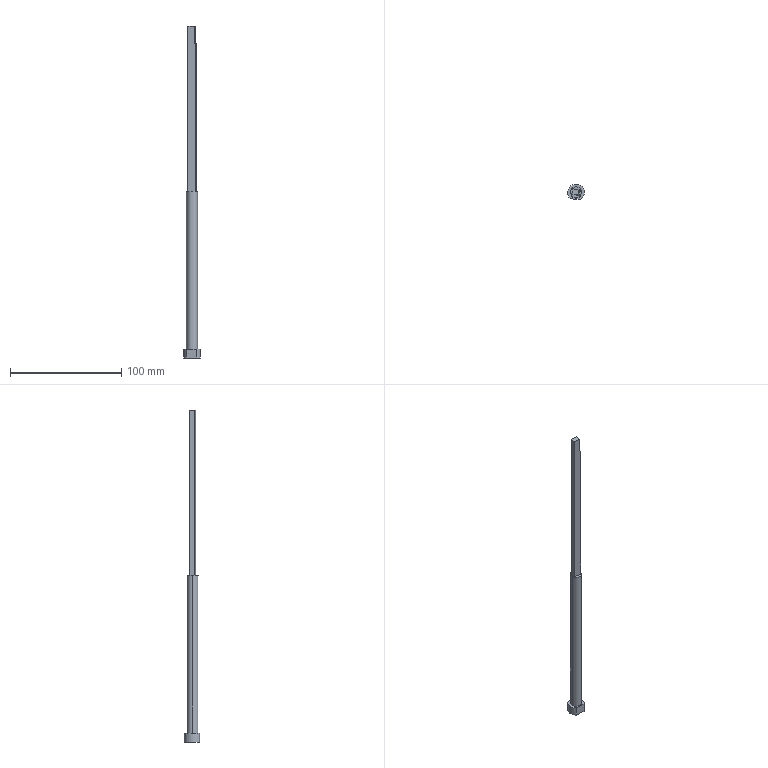Part | Creo | 1 solid | 14 faces | box 15 x 13.938 x 298.951 mm | volume 17637 mm3 | plane 10 | cylinder 3 | cone 1 | commonest cylinder face diameters 10 x2 15 x1
STEP:
#1=CARTESIAN_POINT('',(-71.051,51.227,-12.688));
#2=VERTEX_POINT('',#1);
#3=CARTESIAN_POINT('',(-71.051,51.227,-146.));
#4=VERTEX_POINT('',#3);
#5=CARTESIAN_POINT('',(-71.051,51.227,-12.688));
#6=DIRECTION('',(0.,0.,-1.));
#7=VECTOR('',#6,133.312);
#8=LINE('',#5,#7);
#9=EDGE_CURVE('',#2,#4,#8,.T.);
#10=ORIENTED_EDGE('',*,*,#9,.F.);
#11=CARTESIAN_POINT('',(-70.529,56.199,-12.688));
#12=VERTEX_POINT('',#11);
#13=CARTESIAN_POINT('',(-71.051,51.227,-12.688));
#14=DIRECTION('',(0.1045,0.9945,0.));
#15=VECTOR('',#14,5.);
#16=LINE('',#13,#15);
#17=EDGE_CURVE('',#2,#12,#16,.T.);
#18=ORIENTED_EDGE('',*,*,#17,.T.);
#19=CARTESIAN_POINT('',(-70.529,56.199,-146.));
#20=VERTEX_POINT('',#19);
#21=CARTESIAN_POINT('',(-70.529,56.199,-12.688));
#22=DIRECTION('',(0.,0.,-1.));
#23=VECTOR('',#22,133.312);
#24=LINE('',#21,#23);
#25=EDGE_CURVE('',#12,#20,#24,.T.);
#26=ORIENTED_EDGE('',*,*,#25,.T.);
#27=CARTESIAN_POINT('',(-70.529,56.199,-146.));
#28=DIRECTION('',(-0.1045,-0.9945,0.));
#29=VECTOR('',#28,5.);
#30=LINE('',#27,#29);
#31=EDGE_CURVE('',#20,#4,#30,.T.);
#32=ORIENTED_EDGE('',*,*,#31,.T.);
#33=EDGE_LOOP('',(#10,#18,#26,#32));
#34=FACE_OUTER_BOUND('',#33,.F.);
#35=CARTESIAN_POINT('',(-70.921,52.47,-35.));
#36=DIRECTION('',(0.9945,-0.1045,0.));
#37=DIRECTION('',(0.,0.,1.));
#38=AXIS2_PLACEMENT_3D('',#35,#36,#37);
#39=PLANE('',#38);
#40=ADVANCED_FACE('',(#34),#39,.T.);
#41=CARTESIAN_POINT('',(-71.854,51.311,-12.688));
#42=VERTEX_POINT('',#41);
#43=CARTESIAN_POINT('',(-72.124,51.34,2.9));
#44=VERTEX_POINT('',#43);
#45=CARTESIAN_POINT('',(-71.854,51.311,-12.688));
#46=DIRECTION('',(-0.01736,0.001825,0.9998));
#47=VECTOR('',#46,15.59);
#48=LINE('',#45,#47);
#49=EDGE_CURVE('',#42,#44,#48,.T.);
#50=ORIENTED_EDGE('',*,*,#49,.F.);
#51=CARTESIAN_POINT('',(-71.854,51.311,-12.688));
#52=DIRECTION('',(0.9945,-0.1045,-0.000006119));
#53=VECTOR('',#52,0.807);
#54=LINE('',#51,#53);
#55=EDGE_CURVE('',#42,#2,#54,.T.);
#56=ORIENTED_EDGE('',*,*,#55,.T.);
#57=ORIENTED_EDGE('',*,*,#9,.T.);
#58=CARTESIAN_POINT('',(-78.013,51.958,-146.));
#59=VERTEX_POINT('',#58);
#60=CARTESIAN_POINT('',(-71.051,51.227,-146.));
#61=DIRECTION('',(-0.9945,0.1045,0.));
#62=VECTOR('',#61,7.);
#63=LINE('',#60,#62);
#64=EDGE_CURVE('',#4,#59,#63,.T.);
#65=ORIENTED_EDGE('',*,*,#64,.T.);
#66=CARTESIAN_POINT('',(-78.013,51.958,2.951));
#67=VERTEX_POINT('',#66);
#68=CARTESIAN_POINT('',(-78.013,51.958,2.951));
#69=DIRECTION('',(0.,0.,-1.));
#70=VECTOR('',#69,148.951);
#71=LINE('',#68,#70);
#72=EDGE_CURVE('',#67,#59,#71,.T.);
#73=ORIENTED_EDGE('',*,*,#72,.F.);
#74=CARTESIAN_POINT('',(-78.013,51.958,2.951));
#75=DIRECTION('',(0.9945,-0.1045,-0.008677));
#76=VECTOR('',#75,5.921);
#77=LINE('',#74,#76);
#78=EDGE_CURVE('',#67,#44,#77,.T.);
#79=ORIENTED_EDGE('',*,*,#78,.T.);
#80=EDGE_LOOP('',(#50,#56,#57,#65,#73,#79));
#81=FACE_OUTER_BOUND('',#80,.F.);
#82=CARTESIAN_POINT('',(-75.775,51.723,-35.));
#83=DIRECTION('',(-0.1045,-0.9945,0.));
#84=DIRECTION('',(0.,0.,1.));
#85=AXIS2_PLACEMENT_3D('',#82,#83,#84);
#86=PLANE('',#85);
#87=ADVANCED_FACE('',(#81),#86,.T.);
#88=CARTESIAN_POINT('',(-71.456,56.297,2.894));
#89=VERTEX_POINT('',#88);
#90=CARTESIAN_POINT('',(-71.185,56.268,-12.688));
#91=VERTEX_POINT('',#90);
#92=CARTESIAN_POINT('',(-71.456,56.297,2.894));
#93=DIRECTION('',(0.01737,-0.001825,-0.9998));
#94=VECTOR('',#93,15.585);
#95=LINE('',#92,#94);
#96=EDGE_CURVE('',#89,#91,#95,.T.);
#97=ORIENTED_EDGE('',*,*,#96,.T.);
#98=CARTESIAN_POINT('',(-71.185,56.268,-12.688));
#99=CARTESIAN_POINT('',(-71.263,55.717,-12.688));
#100=CARTESIAN_POINT('',(-71.417,54.613,-12.688));
#101=CARTESIAN_POINT('',(-71.639,52.961,-12.688));
#102=CARTESIAN_POINT('',(-71.783,51.861,-12.688));
#103=CARTESIAN_POINT('',(-71.854,51.311,-12.688));
#104=B_SPLINE_CURVE_WITH_KNOTS('',3,(#98,#99,#100,#101,#102,#103),.UNSPECIFIED.,.F.,.F.,(4,1,1,4),(0.,0.3333,0.6667,1.),.UNSPECIFIED.);
#105=EDGE_CURVE('',#91,#42,#104,.T.);
#106=ORIENTED_EDGE('',*,*,#105,.T.);
#107=ORIENTED_EDGE('',*,*,#49,.T.);
#108=CARTESIAN_POINT('',(-72.124,51.34,2.9));
#109=CARTESIAN_POINT('',(-72.053,51.891,2.899));
#110=CARTESIAN_POINT('',(-71.91,52.993,2.898));
#111=CARTESIAN_POINT('',(-71.687,54.646,2.896));
#112=CARTESIAN_POINT('',(-71.533,55.746,2.895));
#113=CARTESIAN_POINT('',(-71.456,56.297,2.894));
#114=B_SPLINE_CURVE_WITH_KNOTS('',3,(#108,#109,#110,#111,#112,#113),.UNSPECIFIED.,.F.,.F.,(4,1,1,4),(0.,0.3333,0.6667,1.),.UNSPECIFIED.);
#115=EDGE_CURVE('',#44,#89,#114,.T.);
#116=ORIENTED_EDGE('',*,*,#115,.T.);
#117=EDGE_LOOP('',(#97,#106,#107,#116));
#118=FACE_OUTER_BOUND('',#117,.F.);
#119=CARTESIAN_POINT('',(344.456,-2.301,-4.943));
#120=DIRECTION('',(0.0001143,-0.00001653,1.));
#121=DIRECTION('',(-0.9902,0.1395,0.0001155));
#122=AXIS2_PLACEMENT_3D('',#119,#120,#121);
#123=CONICAL_SURFACE('',#122,419.883,1.007);
#124=ADVANCED_FACE('',(#118),#123,.F.);
#125=ORIENTED_EDGE('',*,*,#25,.F.);
#126=CARTESIAN_POINT('',(-70.529,56.199,-12.688));
#127=DIRECTION('',(-0.9945,0.1045,0.000007477));
#128=VECTOR('',#127,0.6604);
#129=LINE('',#126,#128);
#130=EDGE_CURVE('',#12,#91,#129,.T.);
#131=ORIENTED_EDGE('',*,*,#130,.T.);
#132=ORIENTED_EDGE('',*,*,#96,.F.);
#133=CARTESIAN_POINT('',(-77.49,56.931,2.947));
#134=VERTEX_POINT('',#133);
#135=CARTESIAN_POINT('',(-71.456,56.297,2.894));
#136=DIRECTION('',(-0.9945,0.1045,0.008678));
#137=VECTOR('',#136,6.068);
#138=LINE('',#135,#137);
#139=EDGE_CURVE('',#89,#134,#138,.T.);
#140=ORIENTED_EDGE('',*,*,#139,.T.);
#141=CARTESIAN_POINT('',(-77.49,56.931,-146.));
#142=VERTEX_POINT('',#141);
#143=CARTESIAN_POINT('',(-77.49,56.931,2.947));
#144=DIRECTION('',(0.,0.,-1.));
#145=VECTOR('',#144,148.947);
#146=LINE('',#143,#145);
#147=EDGE_CURVE('',#134,#142,#146,.T.);
#148=ORIENTED_EDGE('',*,*,#147,.T.);
#149=CARTESIAN_POINT('',(-77.49,56.931,-146.));
#150=DIRECTION('',(0.9945,-0.1045,0.));
#151=VECTOR('',#150,7.);
#152=LINE('',#149,#151);
#153=EDGE_CURVE('',#142,#20,#152,.T.);
#154=ORIENTED_EDGE('',*,*,#153,.T.);
#155=EDGE_LOOP('',(#125,#131,#132,#140,#148,#154));
#156=FACE_OUTER_BOUND('',#155,.F.);
#157=CARTESIAN_POINT('',(-75.253,56.696,-35.));
#158=DIRECTION('',(0.1045,0.9945,0.));
#159=DIRECTION('',(0.,0.,-1.));
#160=AXIS2_PLACEMENT_3D('',#157,#158,#159);
#161=PLANE('',#160);
#162=ADVANCED_FACE('',(#156),#161,.T.);
#163=ORIENTED_EDGE('',*,*,#17,.F.);
#164=ORIENTED_EDGE('',*,*,#55,.F.);
#165=ORIENTED_EDGE('',*,*,#105,.F.);
#166=ORIENTED_EDGE('',*,*,#130,.F.);
#167=EDGE_LOOP('',(#163,#164,#165,#166));
#168=FACE_OUTER_BOUND('',#167,.F.);
#169=CARTESIAN_POINT('',(0.,0.,-12.688));
#170=DIRECTION('',(0.,0.,1.));
#171=DIRECTION('',(0.,-1.,0.));
#172=AXIS2_PLACEMENT_3D('',#169,#170,#171);
#173=PLANE('',#172);
#174=ADVANCED_FACE('',(#168),#173,.T.);
#175=ORIENTED_EDGE('',*,*,#115,.F.);
#176=ORIENTED_EDGE('',*,*,#78,.F.);
#177=CARTESIAN_POINT('',(-77.49,56.931,2.947));
#178=DIRECTION('',(-0.1045,-0.9945,0.0009122));
#179=VECTOR('',#178,5.);
#180=LINE('',#177,#179);
#181=EDGE_CURVE('',#134,#67,#180,.T.);
#182=ORIENTED_EDGE('',*,*,#181,.F.);
#183=ORIENTED_EDGE('',*,*,#139,.F.);
#184=EDGE_LOOP('',(#175,#176,#182,#183));
#185=FACE_OUTER_BOUND('',#184,.F.);
#186=CARTESIAN_POINT('',(-86.668,59.295,3.027));
#187=DIRECTION('',(0.008727,0.,1.));
#188=DIRECTION('',(0.,-1.,0.));
#189=AXIS2_PLACEMENT_3D('',#186,#187,#188);
#190=PLANE('',#189);
#191=ADVANCED_FACE('',(#185),#190,.T.);
#192=ORIENTED_EDGE('',*,*,#147,.F.);
#193=ORIENTED_EDGE('',*,*,#181,.T.);
#194=ORIENTED_EDGE('',*,*,#72,.T.);
#195=CARTESIAN_POINT('',(-78.013,51.958,-146.));
#196=DIRECTION('',(0.1045,0.9945,0.));
#197=VECTOR('',#196,5.);
#198=LINE('',#195,#197);
#199=EDGE_CURVE('',#59,#142,#198,.T.);
#200=ORIENTED_EDGE('',*,*,#199,.T.);
#201=EDGE_LOOP('',(#192,#193,#194,#200));
#202=FACE_OUTER_BOUND('',#201,.F.);
#203=CARTESIAN_POINT('',(-77.882,53.202,-35.));
#204=DIRECTION('',(-0.9945,0.1045,0.));
#205=DIRECTION('',(0.,0.,-1.));
#206=AXIS2_PLACEMENT_3D('',#203,#204,#205);
#207=PLANE('',#206);
#208=ADVANCED_FACE('',(#202),#207,.T.);
#209=CARTESIAN_POINT('',(-69.271,54.079,-146.));
#210=VERTEX_POINT('',#209);
#211=CARTESIAN_POINT('',(-79.271,54.079,-146.));
#212=VERTEX_POINT('',#211);
#213=CARTESIAN_POINT('',(-74.271,54.079,-146.));
#214=DIRECTION('',(0.,0.,1.));
#215=DIRECTION('',(1.,0.,0.));
#216=AXIS2_PLACEMENT_3D('',#213,#214,#215);
#217=CIRCLE('',#216,5.);
#218=EDGE_CURVE('',#210,#212,#217,.T.);
#219=ORIENTED_EDGE('',*,*,#218,.F.);
#220=CARTESIAN_POINT('',(-74.271,54.079,-146.));
#221=DIRECTION('',(0.,0.,1.));
#222=DIRECTION('',(-1.,0.,0.));
#223=AXIS2_PLACEMENT_3D('',#220,#221,#222);
#224=CIRCLE('',#223,5.);
#225=EDGE_CURVE('',#212,#210,#224,.T.);
#226=ORIENTED_EDGE('',*,*,#225,.F.);
#227=EDGE_LOOP('',(#219,#226));
#228=FACE_OUTER_BOUND('',#227,.F.);
#229=ORIENTED_EDGE('',*,*,#199,.F.);
#230=ORIENTED_EDGE('',*,*,#64,.F.);
#231=ORIENTED_EDGE('',*,*,#31,.F.);
#232=ORIENTED_EDGE('',*,*,#153,.F.);
#233=EDGE_LOOP('',(#229,#230,#231,#232));
#234=FACE_BOUND('',#233,.F.);
#235=CARTESIAN_POINT('',(-74.271,54.079,-146.));
#236=DIRECTION('',(0.,0.,1.));
#237=DIRECTION('',(-1.,0.,0.));
#238=AXIS2_PLACEMENT_3D('',#235,#236,#237);
#239=PLANE('',#238);
#240=ADVANCED_FACE('',(#228,#234),#239,.T.);
#241=CARTESIAN_POINT('',(-79.271,54.079,-288.));
#242=VERTEX_POINT('',#241);
#243=CARTESIAN_POINT('',(-69.271,54.079,-288.));
#244=VERTEX_POINT('',#243);
#245=CARTESIAN_POINT('',(-74.271,54.079,-288.));
#246=DIRECTION('',(0.,0.,-1.));
#247=DIRECTION('',(-1.,0.,0.));
#248=AXIS2_PLACEMENT_3D('',#245,#246,#247);
#249=CIRCLE('',#248,5.);
#250=EDGE_CURVE('',#242,#244,#249,.T.);
#251=ORIENTED_EDGE('',*,*,#250,.T.);
#252=CARTESIAN_POINT('',(-69.271,54.079,-288.));
#253=DIRECTION('',(0.,0.,1.));
#254=VECTOR('',#253,142.);
#255=LINE('',#252,#254);
#256=EDGE_CURVE('',#244,#210,#255,.T.);
#257=ORIENTED_EDGE('',*,*,#256,.T.);
#258=ORIENTED_EDGE('',*,*,#218,.T.);
#259=CARTESIAN_POINT('',(-79.271,54.079,-288.));
#260=DIRECTION('',(0.,0.,1.));
#261=VECTOR('',#260,142.);
#262=LINE('',#259,#261);
#263=EDGE_CURVE('',#242,#212,#262,.T.);
#264=ORIENTED_EDGE('',*,*,#263,.F.);
#265=EDGE_LOOP('',(#251,#257,#258,#264));
#266=FACE_OUTER_BOUND('',#265,.F.);
#267=CARTESIAN_POINT('',(-74.271,54.079,-245.));
#268=DIRECTION('',(0.,0.,1.));
#269=DIRECTION('',(-1.,0.,0.));
#270=AXIS2_PLACEMENT_3D('',#267,#268,#269);
#271=CYLINDRICAL_SURFACE('',#270,5.);
#272=ADVANCED_FACE('',(#266),#271,.T.);
#273=CARTESIAN_POINT('',(-70.422,47.641,-288.));
#274=VERTEX_POINT('',#273);
#275=CARTESIAN_POINT('',(-66.771,54.079,-288.));
#276=VERTEX_POINT('',#275);
#277=CARTESIAN_POINT('',(-74.271,54.079,-288.));
#278=DIRECTION('',(0.,0.,1.));
#279=DIRECTION('',(0.5131,-0.8583,0.));
#280=AXIS2_PLACEMENT_3D('',#277,#278,#279);
#281=CIRCLE('',#280,7.5);
#282=EDGE_CURVE('',#274,#276,#281,.T.);
#283=ORIENTED_EDGE('',*,*,#282,.F.);
#284=CARTESIAN_POINT('',(-79.373,48.582,-288.));
#285=VERTEX_POINT('',#284);
#286=CARTESIAN_POINT('',(-79.373,48.582,-288.));
#287=DIRECTION('',(0.9945,-0.1045,0.));
#288=VECTOR('',#287,9.);
#289=LINE('',#286,#288);
#290=EDGE_CURVE('',#285,#274,#289,.T.);
#291=ORIENTED_EDGE('',*,*,#290,.F.);
#292=CARTESIAN_POINT('',(-74.271,54.079,-288.));
#293=DIRECTION('',(0.,0.,1.));
#294=DIRECTION('',(1.,0.,0.));
#295=AXIS2_PLACEMENT_3D('',#292,#293,#294);
#296=CIRCLE('',#295,7.5);
#297=EDGE_CURVE('',#276,#285,#296,.T.);
#298=ORIENTED_EDGE('',*,*,#297,.F.);
#299=EDGE_LOOP('',(#283,#291,#298));
#300=FACE_OUTER_BOUND('',#299,.F.);
#301=ORIENTED_EDGE('',*,*,#250,.F.);
#302=CARTESIAN_POINT('',(-74.271,54.079,-288.));
#303=DIRECTION('',(0.,0.,-1.));
#304=DIRECTION('',(1.,0.,0.));
#305=AXIS2_PLACEMENT_3D('',#302,#303,#304);
#306=CIRCLE('',#305,5.);
#307=EDGE_CURVE('',#244,#242,#306,.T.);
#308=ORIENTED_EDGE('',*,*,#307,.F.);
#309=EDGE_LOOP('',(#301,#308));
#310=FACE_BOUND('',#309,.F.);
#311=CARTESIAN_POINT('',(-47.,-35.,-288.));
#312=DIRECTION('',(0.,0.,-1.));
#313=DIRECTION('',(1.,0.,0.));
#314=AXIS2_PLACEMENT_3D('',#311,#312,#313);
#315=PLANE('',#314);
#316=ADVANCED_FACE('',(#300,#310),#315,.F.);
#317=ORIENTED_EDGE('',*,*,#307,.T.);
#318=ORIENTED_EDGE('',*,*,#263,.T.);
#319=ORIENTED_EDGE('',*,*,#225,.T.);
#320=ORIENTED_EDGE('',*,*,#256,.F.);
#321=EDGE_LOOP('',(#317,#318,#319,#320));
#322=FACE_OUTER_BOUND('',#321,.F.);
#323=CARTESIAN_POINT('',(-74.271,54.079,-245.));
#324=DIRECTION('',(0.,0.,1.));
#325=DIRECTION('',(-1.,0.,0.));
#326=AXIS2_PLACEMENT_3D('',#323,#324,#325);
#327=CYLINDRICAL_SURFACE('',#326,5.);
#328=ADVANCED_FACE('',(#322),#327,.T.);
#329=CARTESIAN_POINT('',(-70.422,47.641,-296.));
#330=VERTEX_POINT('',#329);
#331=CARTESIAN_POINT('',(-70.422,47.641,-288.));
#332=DIRECTION('',(0.,0.,-1.));
#333=VECTOR('',#332,8.);
#334=LINE('',#331,#333);
#335=EDGE_CURVE('',#274,#330,#334,.T.);
#336=ORIENTED_EDGE('',*,*,#335,.F.);
#337=ORIENTED_EDGE('',*,*,#282,.T.);
#338=ORIENTED_EDGE('',*,*,#297,.T.);
#339=CARTESIAN_POINT('',(-79.373,48.582,-296.));
#340=VERTEX_POINT('',#339);
#341=CARTESIAN_POINT('',(-79.373,48.582,-296.));
#342=DIRECTION('',(0.,0.,1.));
#343=VECTOR('',#342,8.);
#344=LINE('',#341,#343);
#345=EDGE_CURVE('',#340,#285,#344,.T.);
#346=ORIENTED_EDGE('',*,*,#345,.F.);
#347=CARTESIAN_POINT('',(-66.771,54.079,-296.));
#348=VERTEX_POINT('',#347);
#349=CARTESIAN_POINT('',(-74.271,54.079,-296.));
#350=DIRECTION('',(0.,0.,-1.));
#351=DIRECTION('',(-0.6803,-0.7329,0.));
#352=AXIS2_PLACEMENT_3D('',#349,#350,#351);
#353=CIRCLE('',#352,7.5);
#354=EDGE_CURVE('',#340,#348,#353,.T.);
#355=ORIENTED_EDGE('',*,*,#354,.T.);
#356=CARTESIAN_POINT('',(-74.271,54.079,-296.));
#357=DIRECTION('',(0.,0.,-1.));
#358=DIRECTION('',(1.,0.,0.));
#359=AXIS2_PLACEMENT_3D('',#356,#357,#358);
#360=CIRCLE('',#359,7.5);
#361=EDGE_CURVE('',#348,#330,#360,.T.);
#362=ORIENTED_EDGE('',*,*,#361,.T.);
#363=EDGE_LOOP('',(#336,#337,#338,#346,#355,#362));
#364=FACE_OUTER_BOUND('',#363,.F.);
#365=CARTESIAN_POINT('',(-74.271,54.079,-288.));
#366=DIRECTION('',(0.,0.,-1.));
#367=DIRECTION('',(1.,0.,0.));
#368=AXIS2_PLACEMENT_3D('',#365,#366,#367);
#369=CYLINDRICAL_SURFACE('',#368,7.5);
#370=ADVANCED_FACE('',(#364),#369,.T.);
#371=ORIENTED_EDGE('',*,*,#290,.T.);
#372=ORIENTED_EDGE('',*,*,#335,.T.);
#373=CARTESIAN_POINT('',(-70.422,47.641,-296.));
#374=DIRECTION('',(-0.9945,0.1045,0.));
#375=VECTOR('',#374,9.);
#376=LINE('',#373,#375);
#377=EDGE_CURVE('',#330,#340,#376,.T.);
#378=ORIENTED_EDGE('',*,*,#377,.T.);
#379=ORIENTED_EDGE('',*,*,#345,.T.);
#380=EDGE_LOOP('',(#371,#372,#378,#379));
#381=FACE_OUTER_BOUND('',#380,.F.);
#382=CARTESIAN_POINT('',(-74.898,48.112,-70.026));
#383=DIRECTION('',(-0.1045,-0.9945,0.));
#384=DIRECTION('',(0.9945,-0.1045,0.));
#385=AXIS2_PLACEMENT_3D('',#382,#383,#384);
#386=PLANE('',#385);
#387=ADVANCED_FACE('',(#381),#386,.T.);
#388=ORIENTED_EDGE('',*,*,#377,.F.);
#389=ORIENTED_EDGE('',*,*,#361,.F.);
#390=ORIENTED_EDGE('',*,*,#354,.F.);
#391=EDGE_LOOP('',(#388,#389,#390));
#392=FACE_OUTER_BOUND('',#391,.F.);
#393=CARTESIAN_POINT('',(-47.,-35.,-296.));
#394=DIRECTION('',(0.,0.,-1.));
#395=DIRECTION('',(1.,0.,0.));
#396=AXIS2_PLACEMENT_3D('',#393,#394,#395);
#397=PLANE('',#396);
#398=ADVANCED_FACE('',(#392),#397,.T.);
#399=CLOSED_SHELL('',(#40,#87,#124,#162,#174,#191,#208,#240,#272,#316,#328,#370,#387,#398));
#400=MANIFOLD_SOLID_BREP('',#399);
#401=(LENGTH_UNIT()NAMED_UNIT(*)SI_UNIT(.MILLI.,.METRE.));
#402=UNCERTAINTY_MEASURE_WITH_UNIT(LENGTH_MEASURE(0.02996),#401,'','');
#403=(NAMED_UNIT(*)PLANE_ANGLE_UNIT()SI_UNIT($,.RADIAN.));
#404=PLANE_ANGLE_MEASURE_WITH_UNIT(PLANE_ANGLE_MEASURE(0.01745),#403);
#405=(CONVERSION_BASED_UNIT('DEGREE',#404)NAMED_UNIT(*)PLANE_ANGLE_UNIT());
#406=(NAMED_UNIT(*)SI_UNIT($,.STERADIAN.)SOLID_ANGLE_UNIT());
#407=(GEOMETRIC_REPRESENTATION_CONTEXT(3)GLOBAL_UNCERTAINTY_ASSIGNED_CONTEXT((#402))GLOBAL_UNIT_ASSIGNED_CONTEXT((#401,#405,#406))REPRESENTATION_CONTEXT('',''));
#408=ADVANCED_BREP_SHAPE_REPRESENTATION('',(#400),#407);